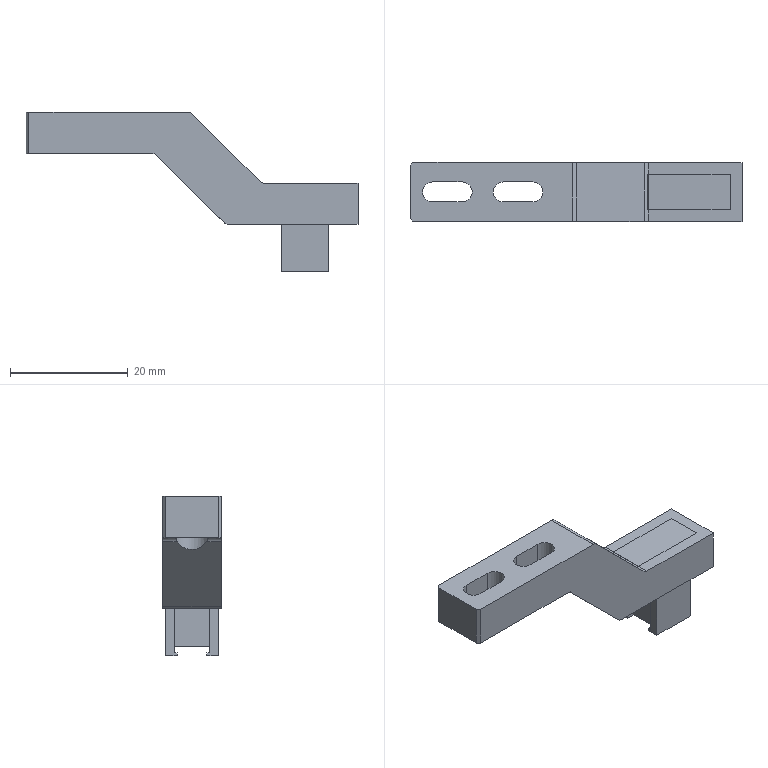NC program | NX | posted with a generic post | part box 56.3 x 10 x 27 mm
Lines 2775 to 3642 of 5717:
(ZLEVEL_PROFILE_COPY_2 , TOOL : D2)
N5506 T02 M6
N5508 G54
N5510 G17 G0 G90 X-11.938 Y0.7 S9500 M3
N5512 G43 Z30. H2
N5514 Z1.5
N5516 G94 G1 X-12.439 Z1.474 F800.
N5518 X-12.69 Y0.606 Z1.46
N5520 X-12.889 Y0.425 Z1.446
N5522 X-12.997 Y0.214 Z1.433
N5524 X-13.025 Y-0.086 Z1.417
N5526 X-12.926 Y-0.37 Z1.402
N5528 X-12.718 Y-0.588 Z1.386
N5530 X-12.439 Y-0.7 Z1.37
N5532 X-7.244 Z1.098
N5534 X-7.053 Y-0.658 Z1.088
N5536 X-6.815 Y-0.499 Z1.073
N5538 X-6.659 Y-0.259 Z1.058
N5540 X-6.611 Y0.023 Z1.043
N5542 X-6.678 Y0.302 Z1.028
N5544 X-6.813 Y0.497 Z1.015
N5546 X-6.991 Y0.629 Z1.003
N5548 X-7.202 Y0.7 Z0.992
N5550 X-12.439 Z0.717
N5552 X-12.69 Y0.606 Z0.703
N5554 X-12.889 Y0.425 Z0.689
N5556 X-12.997 Y0.214 Z0.677
N5558 X-13.025 Y-0.086 Z0.661
N5560 X-12.926 Y-0.37 Z0.645
N5562 X-12.718 Y-0.588 Z0.629
N5564 X-12.439 Y-0.7 Z0.614
N5566 X-7.244 Z0.341
N5568 X-7.053 Y-0.658 Z0.331
N5570 X-6.815 Y-0.499 Z0.316
N5572 X-6.659 Y-0.259 Z0.301
N5574 X-6.611 Y0.023 Z0.286
N5576 X-6.678 Y0.302 Z0.271
N5578 X-6.813 Y0.497 Z0.259
N5580 X-6.991 Y0.629 Z0.247
N5582 X-7.202 Y0.7 Z0.235
N5584 X-12.439 Z-0.039
N5586 X-12.69 Y0.606 Z-0.053
N5588 X-12.889 Y0.425 Z-0.067
N5590 X-12.997 Y0.214 Z-0.08
N5592 X-13.025 Y-0.086 Z-0.095
N5594 X-12.926 Y-0.37 Z-0.111
N5596 X-12.718 Y-0.588 Z-0.127
N5598 X-12.439 Y-0.7 Z-0.143
N5600 X-12.32 Z-0.149
N5602 X-7.32 F1100.
N5604 G3 X-6.62 Y0. R0.7
N5606 X-7.32 Y0.7 R0.7
N5608 G1 X-12.32
N5610 G3 X-13.02 Y0. R0.7
N5612 X-12.32 Y-0.7 R0.7
N5614 G1 X-7.359 Z-0.236
N5616 X-7.226 Y-0.686 Z-0.238
N5618 X-7.164 Y-0.676 Z-0.239
N5620 X-7.061 Y-0.643 Z-0.241
N5622 X-6.982 Y-0.604 Z-0.242
N5624 X-6.888 Y-0.541 Z-0.244
N5626 X-6.826 Y-0.485 Z-0.246
N5628 X-6.755 Y-0.399 Z-0.248
N5630 X-6.709 Y-0.328 Z-0.249
N5632 X-6.656 Y-0.221 Z-0.251
N5634 X-6.636 Y-0.146 Z-0.253
N5636 X-6.622 Y0.052 Z-0.256
N5638 X-6.642 Y0.173 Z-0.258
N5640 X-6.671 Y0.242 Z-0.26
N5642 X-6.735 Y0.373 Z-0.262
N5644 X-6.765 Y0.414 Z-0.263
N5646 X-6.853 Y0.511 Z-0.266
N5648 X-6.902 Y0.554 Z-0.267
N5650 X-6.994 Y0.612 Z-0.269
N5652 X-7.074 Y0.647 Z-0.27
N5654 X-7.161 Y0.675 Z-0.272
N5656 X-7.265 Y0.69 Z-0.274
N5658 X-7.364 Y0.7 Z-0.275
N5660 X-7.463 Z-0.277
N5662 X-8.654 Z-0.298
N5664 X-12.32
N5666 G3 X-13.02 Y0. R0.7
N5668 X-12.32 Y-0.7 R0.7
N5670 G1 X-7.359 Z-0.384
N5672 X-7.226 Y-0.686 Z-0.387
N5674 X-7.164 Y-0.676 Z-0.388
N5676 X-7.061 Y-0.643 Z-0.39
N5678 X-6.982 Y-0.604 Z-0.391
N5680 X-6.888 Y-0.541 Z-0.393
N5682 X-6.826 Y-0.485 Z-0.395
N5684 X-6.755 Y-0.399 Z-0.397
N5686 X-6.709 Y-0.328 Z-0.398
N5688 X-6.656 Y-0.221 Z-0.4
N5690 X-6.636 Y-0.146 Z-0.402
N5692 X-6.622 Y0.052 Z-0.405
N5694 X-6.642 Y0.173 Z-0.407
N5696 X-6.671 Y0.242 Z-0.409
N5698 X-6.735 Y0.373 Z-0.411
N5700 X-6.765 Y0.414 Z-0.412
N5702 X-6.853 Y0.511 Z-0.414
N5704 X-6.902 Y0.554 Z-0.416
N5706 X-6.994 Y0.612 Z-0.418
N5708 X-7.074 Y0.647 Z-0.419
N5710 X-7.161 Y0.675 Z-0.421
N5712 X-7.265 Y0.69 Z-0.423
N5714 X-7.364 Y0.7 Z-0.424
N5716 X-7.463 Z-0.426
N5718 X-8.654 Z-0.447
N5720 X-12.32
N5722 G3 X-13.02 Y0. R0.7
N5724 X-12.32 Y-0.7 R0.7
N5726 G1 X-7.359 Z-0.533
N5728 X-7.226 Y-0.686 Z-0.536
N5730 X-7.164 Y-0.676 Z-0.537
N5732 X-7.061 Y-0.643 Z-0.539
N5734 X-6.982 Y-0.604 Z-0.54
N5736 X-6.888 Y-0.541 Z-0.542
N5738 X-6.826 Y-0.485 Z-0.544
N5740 X-6.755 Y-0.399 Z-0.546
N5742 X-6.709 Y-0.328 Z-0.547
N5744 X-6.656 Y-0.221 Z-0.549
N5746 X-6.636 Y-0.146 Z-0.551
N5748 X-6.622 Y0.052 Z-0.554
N5750 X-6.642 Y0.173 Z-0.556
N5752 X-6.671 Y0.242 Z-0.558
N5754 X-6.735 Y0.373 Z-0.56
N5756 X-6.765 Y0.414 Z-0.561
N5758 X-6.853 Y0.511 Z-0.563
N5760 X-6.902 Y0.554 Z-0.565
N5762 X-6.994 Y0.612 Z-0.566
N5764 X-7.074 Y0.647 Z-0.568
N5766 X-7.161 Y0.675 Z-0.57
N5768 X-7.265 Y0.69 Z-0.572
N5770 X-7.364 Y0.7 Z-0.573
N5772 X-7.463 Z-0.575
N5774 X-8.654 Z-0.596
N5776 X-12.32
N5778 G3 X-13.02 Y0. R0.7
N5780 X-12.32 Y-0.7 R0.7
N5782 G1 X-7.359 Z-0.682
N5784 X-7.226 Y-0.686 Z-0.685
N5786 X-7.164 Y-0.676 Z-0.686
N5788 X-7.061 Y-0.643 Z-0.688
N5790 X-6.982 Y-0.604 Z-0.689
N5792 X-6.888 Y-0.541 Z-0.691
N5794 X-6.826 Y-0.485 Z-0.693
N5796 X-6.755 Y-0.399 Z-0.695
N5798 X-6.709 Y-0.328 Z-0.696
N5800 X-6.656 Y-0.221 Z-0.698
N5802 X-6.636 Y-0.146 Z-0.7
N5804 X-6.622 Y0.052 Z-0.703
N5806 X-6.642 Y0.173 Z-0.705
N5808 X-6.671 Y0.242 Z-0.707
N5810 X-6.735 Y0.373 Z-0.709
N5812 X-6.765 Y0.414 Z-0.71
N5814 X-6.853 Y0.511 Z-0.712
N5816 X-6.902 Y0.554 Z-0.714
N5818 X-6.994 Y0.612 Z-0.715
N5820 X-7.074 Y0.647 Z-0.717
N5822 X-7.161 Y0.675 Z-0.719
N5824 X-7.265 Y0.69 Z-0.72
N5826 X-7.364 Y0.7 Z-0.722
N5828 X-7.463 Z-0.724
N5830 X-8.654 Z-0.745
N5832 X-12.32
N5834 G3 X-13.02 Y0. R0.7
N5836 X-12.32 Y-0.7 R0.7
N5838 G1 X-7.359 Z-0.831
N5840 X-7.226 Y-0.686 Z-0.834
N5842 X-7.164 Y-0.676 Z-0.835
N5844 X-7.061 Y-0.643 Z-0.837
N5846 X-6.982 Y-0.604 Z-0.838
N5848 X-6.888 Y-0.541 Z-0.84
N5850 X-6.826 Y-0.485 Z-0.842
N5852 X-6.755 Y-0.399 Z-0.844
N5854 X-6.709 Y-0.328 Z-0.845
N5856 X-6.656 Y-0.221 Z-0.847
N5858 X-6.636 Y-0.146 Z-0.849
N5860 X-6.622 Y0.052 Z-0.852
N5862 X-6.642 Y0.173 Z-0.854
N5864 X-6.671 Y0.242 Z-0.856
N5866 X-6.735 Y0.373 Z-0.858
N5868 X-6.765 Y0.414 Z-0.859
N5870 X-6.853 Y0.511 Z-0.861
N5872 X-6.902 Y0.554 Z-0.862
N5874 X-6.994 Y0.612 Z-0.864
N5876 X-7.074 Y0.647 Z-0.866
N5878 X-7.161 Y0.675 Z-0.868
N5880 X-7.265 Y0.69 Z-0.869
N5882 X-7.364 Y0.7 Z-0.871
N5884 X-7.463 Z-0.873
N5886 X-8.654 Z-0.894
N5888 X-12.32
N5890 G3 X-13.02 Y0. R0.7
N5892 X-12.32 Y-0.7 R0.7
N5894 G1 X-7.359 Z-0.98
N5896 X-7.226 Y-0.686 Z-0.983
N5898 X-7.164 Y-0.676 Z-0.984
N5900 X-7.061 Y-0.643 Z-0.986
N5902 X-6.982 Y-0.604 Z-0.987
N5904 X-6.888 Y-0.541 Z-0.989
N5906 X-6.826 Y-0.485 Z-0.991
N5908 X-6.755 Y-0.399 Z-0.993
N5910 X-6.709 Y-0.328 Z-0.994
N5912 X-6.656 Y-0.221 Z-0.996
N5914 X-6.636 Y-0.146 Z-0.998
N5916 X-6.622 Y0.052 Z-1.001
N5918 X-6.642 Y0.173 Z-1.003
N5920 X-6.671 Y0.242 Z-1.004
N5922 X-6.735 Y0.373 Z-1.007
N5924 X-6.765 Y0.414 Z-1.008
N5926 X-6.853 Y0.511 Z-1.01
N5928 X-6.902 Y0.554 Z-1.011
N5930 X-6.994 Y0.612 Z-1.013
N5932 X-7.074 Y0.647 Z-1.015
N5934 X-7.161 Y0.675 Z-1.016
N5936 X-7.265 Y0.69 Z-1.018
N5938 X-7.364 Y0.7 Z-1.02
N5940 X-7.463 Z-1.022
N5942 X-8.654 Z-1.043
N5944 X-12.32
N5946 G3 X-13.02 Y0. R0.7
N5948 X-12.32 Y-0.7 R0.7
N5950 G1 X-7.359 Z-1.129
N5952 X-7.226 Y-0.686 Z-1.131
N5954 X-7.164 Y-0.676 Z-1.133
N5956 X-7.061 Y-0.643 Z-1.135
N5958 X-6.982 Y-0.604 Z-1.136
N5960 X-6.888 Y-0.541 Z-1.138
N5962 X-6.826 Y-0.485 Z-1.14
N5964 X-6.755 Y-0.399 Z-1.142
N5966 X-6.709 Y-0.328 Z-1.143
N5968 X-6.656 Y-0.221 Z-1.145
N5970 X-6.636 Y-0.146 Z-1.146
N5972 X-6.622 Y0.052 Z-1.15
N5974 X-6.642 Y0.173 Z-1.152
N5976 X-6.671 Y0.242 Z-1.153
N5978 X-6.735 Y0.373 Z-1.156
N5980 X-6.765 Y0.414 Z-1.157
N5982 X-6.853 Y0.511 Z-1.159
N5984 X-6.902 Y0.554 Z-1.16
N5986 X-6.994 Y0.612 Z-1.162
N5988 X-7.074 Y0.647 Z-1.164
N5990 X-7.161 Y0.675 Z-1.165
N5992 X-7.265 Y0.69 Z-1.167
N5994 X-7.364 Y0.7 Z-1.169
N5996 X-7.463 Z-1.171
N5998 X-8.654 Z-1.191
N6000 X-12.32
N6002 G3 X-13.02 Y0. R0.7
N6004 X-12.32 Y-0.7 R0.7
N6006 G1 X-7.359 Z-1.278
N6008 X-7.226 Y-0.686 Z-1.28
N6010 X-7.164 Y-0.676 Z-1.282
N6012 X-7.061 Y-0.643 Z-1.283
N6014 X-6.982 Y-0.604 Z-1.285
N6016 X-6.888 Y-0.541 Z-1.287
N6018 X-6.826 Y-0.485 Z-1.288
N6020 X-6.755 Y-0.399 Z-1.29
N6022 X-6.709 Y-0.328 Z-1.292
N6024 X-6.656 Y-0.221 Z-1.294
N6026 X-6.636 Y-0.146 Z-1.295
N6028 X-6.622 Y0.052 Z-1.299
N6030 X-6.642 Y0.173 Z-1.301
N6032 X-6.671 Y0.242 Z-1.302
N6034 X-6.735 Y0.373 Z-1.305
N6036 X-6.765 Y0.414 Z-1.306
N6038 X-6.853 Y0.511 Z-1.308
N6040 X-6.902 Y0.554 Z-1.309
N6042 X-6.994 Y0.612 Z-1.311
N6044 X-7.074 Y0.647 Z-1.313
N6046 X-7.161 Y0.675 Z-1.314
N6048 X-7.265 Y0.69 Z-1.316
N6050 X-7.364 Y0.7 Z-1.318
N6052 X-7.463 Z-1.32
N6054 X-8.654 Z-1.34
N6056 X-12.32
N6058 G3 X-13.02 Y0. R0.7
N6060 X-12.32 Y-0.7 R0.7
N6062 G1 X-7.359 Z-1.427
N6064 X-7.226 Y-0.686 Z-1.429
N6066 X-7.164 Y-0.676 Z-1.43
N6068 X-7.061 Y-0.643 Z-1.432
N6070 X-6.982 Y-0.604 Z-1.434
N6072 X-6.888 Y-0.541 Z-1.436
N6074 X-6.826 Y-0.485 Z-1.437
N6076 X-6.755 Y-0.399 Z-1.439
N6078 X-6.709 Y-0.328 Z-1.441
N6080 X-6.656 Y-0.221 Z-1.443
N6082 X-6.636 Y-0.146 Z-1.444
N6084 X-6.622 Y0.052 Z-1.448
N6086 X-6.642 Y0.173 Z-1.45
N6088 X-6.671 Y0.242 Z-1.451
N6090 X-6.735 Y0.373 Z-1.454
N6092 X-6.765 Y0.414 Z-1.455
N6094 X-6.853 Y0.511 Z-1.457
N6096 X-6.902 Y0.554 Z-1.458
N6098 X-6.994 Y0.612 Z-1.46
N6100 X-7.074 Y0.647 Z-1.462
N6102 X-7.161 Y0.675 Z-1.463
N6104 X-7.265 Y0.69 Z-1.465
N6106 X-7.364 Y0.7 Z-1.467
N6108 X-7.463 Z-1.469
N6110 X-8.654 Z-1.489
N6112 X-12.32
N6114 G3 X-13.02 Y0. R0.7
N6116 X-12.32 Y-0.7 R0.7
N6118 G1 X-7.359 Z-1.576
N6120 X-7.226 Y-0.686 Z-1.578
N6122 X-7.164 Y-0.676 Z-1.579
N6124 X-7.061 Y-0.643 Z-1.581
N6126 X-6.982 Y-0.604 Z-1.583
N6128 X-6.888 Y-0.541 Z-1.585
N6130 X-6.826 Y-0.485 Z-1.586
N6132 X-6.755 Y-0.399 Z-1.588
N6134 X-6.709 Y-0.328 Z-1.59
N6136 X-6.656 Y-0.221 Z-1.592
N6138 X-6.636 Y-0.146 Z-1.593
N6140 X-6.622 Y0.052 Z-1.597
N6142 X-6.642 Y0.173 Z-1.599
N6144 X-6.671 Y0.242 Z-1.6
N6146 X-6.735 Y0.373 Z-1.603
N6148 X-6.765 Y0.414 Z-1.604
N6150 X-6.853 Y0.511 Z-1.606
N6152 X-6.902 Y0.554 Z-1.607
N6154 X-6.994 Y0.612 Z-1.609
N6156 X-7.074 Y0.647 Z-1.611
N6158 X-7.161 Y0.675 Z-1.612
N6160 X-7.265 Y0.69 Z-1.614
N6162 X-7.364 Y0.7 Z-1.616
N6164 X-7.463 Z-1.618
N6166 X-8.654 Z-1.638
N6168 X-12.32
N6170 G3 X-13.02 Y0. R0.7
N6172 X-12.32 Y-0.7 R0.7
N6174 G1 X-7.359 Z-1.725
N6176 X-7.226 Y-0.686 Z-1.727
N6178 X-7.164 Y-0.676 Z-1.728
N6180 X-7.061 Y-0.643 Z-1.73
N6182 X-6.982 Y-0.604 Z-1.732
N6184 X-6.888 Y-0.541 Z-1.734
N6186 X-6.826 Y-0.485 Z-1.735
N6188 X-6.755 Y-0.399 Z-1.737
N6190 X-6.709 Y-0.328 Z-1.739
N6192 X-6.656 Y-0.221 Z-1.741
N6194 X-6.636 Y-0.146 Z-1.742
N6196 X-6.622 Y0.052 Z-1.746
N6198 X-6.642 Y0.173 Z-1.748
N6200 X-6.671 Y0.242 Z-1.749
N6202 X-6.735 Y0.373 Z-1.752
N6204 X-6.765 Y0.414 Z-1.753
N6206 X-6.853 Y0.511 Z-1.755
N6208 X-6.902 Y0.554 Z-1.756
N6210 X-6.994 Y0.612 Z-1.758
N6212 X-7.074 Y0.647 Z-1.76
N6214 X-7.161 Y0.675 Z-1.761
N6216 X-7.265 Y0.69 Z-1.763
N6218 X-7.364 Y0.7 Z-1.765
N6220 X-7.463 Z-1.766
N6222 X-8.654 Z-1.787
N6224 X-12.32
N6226 G3 X-13.02 Y0. R0.7
N6228 X-12.32 Y-0.7 R0.7
N6230 G1 X-7.359 Z-1.874
N6232 X-7.226 Y-0.686 Z-1.876
N6234 X-7.164 Y-0.676 Z-1.877
N6236 X-7.061 Y-0.643 Z-1.879
N6238 X-6.982 Y-0.604 Z-1.881
N6240 X-6.888 Y-0.541 Z-1.883
N6242 X-6.826 Y-0.485 Z-1.884
N6244 X-6.755 Y-0.399 Z-1.886
N6246 X-6.709 Y-0.328 Z-1.888
N6248 X-6.656 Y-0.221 Z-1.89
N6250 X-6.636 Y-0.146 Z-1.891
N6252 X-6.622 Y0.052 Z-1.895
N6254 X-6.642 Y0.173 Z-1.897
N6256 X-6.671 Y0.242 Z-1.898
N6258 X-6.735 Y0.373 Z-1.901
N6260 X-6.765 Y0.414 Z-1.902
N6262 X-6.853 Y0.511 Z-1.904
N6264 X-6.902 Y0.554 Z-1.905
N6266 X-6.994 Y0.612 Z-1.907
N6268 X-7.074 Y0.647 Z-1.908
N6270 X-7.161 Y0.675 Z-1.91
N6272 X-7.265 Y0.69 Z-1.912
N6274 X-7.364 Y0.7 Z-1.914
N6276 X-7.463 Z-1.915
N6278 X-8.654 Z-1.936
N6280 X-12.32
N6282 G3 X-13.02 Y0. R0.7
N6284 X-12.32 Y-0.7 R0.7
N6286 G1 X-7.359 Z-2.023
N6288 X-7.226 Y-0.686 Z-2.025
N6290 X-7.164 Y-0.676 Z-2.026
N6292 X-7.061 Y-0.643 Z-2.028
N6294 X-6.982 Y-0.604 Z-2.03
N6296 X-6.888 Y-0.541 Z-2.032
N6298 X-6.826 Y-0.485 Z-2.033
N6300 X-6.755 Y-0.399 Z-2.035
N6302 X-6.709 Y-0.328 Z-2.037
N6304 X-6.656 Y-0.221 Z-2.039
N6306 X-6.636 Y-0.146 Z-2.04
N6308 X-6.622 Y0.052 Z-2.044
N6310 X-6.642 Y0.173 Z-2.046
N6312 X-6.671 Y0.242 Z-2.047
N6314 X-6.735 Y0.373 Z-2.05
N6316 X-6.765 Y0.414
N6318 X-6.853 Y0.511 Z-2.053
N6320 X-6.902 Y0.554 Z-2.054
N6322 X-6.994 Y0.612 Z-2.056
N6324 X-7.074 Y0.647 Z-2.057
N6326 X-7.161 Y0.675 Z-2.059
N6328 X-7.265 Y0.69 Z-2.061
N6330 X-7.364 Y0.7 Z-2.063
N6332 X-7.463 Z-2.064
N6334 X-8.654 Z-2.085
N6336 X-12.32
N6338 G3 X-13.02 Y0. R0.7
N6340 X-12.32 Y-0.7 R0.7
N6342 G1 X-7.359 Z-2.172
N6344 X-7.226 Y-0.686 Z-2.174
N6346 X-7.164 Y-0.676 Z-2.175
N6348 X-7.061 Y-0.643 Z-2.177
N6350 X-6.982 Y-0.604 Z-2.179
N6352 X-6.888 Y-0.541 Z-2.181
N6354 X-6.826 Y-0.485 Z-2.182
N6356 X-6.755 Y-0.399 Z-2.184
N6358 X-6.709 Y-0.328 Z-2.186
N6360 X-6.656 Y-0.221 Z-2.188
N6362 X-6.636 Y-0.146 Z-2.189
N6364 X-6.622 Y0.052 Z-2.192
N6366 X-6.642 Y0.173 Z-2.195
N6368 X-6.671 Y0.242 Z-2.196
N6370 X-6.735 Y0.373 Z-2.198
N6372 X-6.765 Y0.414 Z-2.199
N6374 X-6.853 Y0.511 Z-2.202
N6376 X-6.902 Y0.554 Z-2.203
N6378 X-6.994 Y0.612 Z-2.205
N6380 X-7.074 Y0.647 Z-2.206
N6382 X-7.161 Y0.675 Z-2.208
N6384 X-7.265 Y0.69 Z-2.21
N6386 X-7.364 Y0.7 Z-2.212
N6388 X-7.463 Z-2.213
N6390 X-8.654 Z-2.234
N6392 X-12.32
N6394 G3 X-13.02 Y0. R0.7
N6396 X-12.32 Y-0.7 R0.7
N6398 G1 X-7.359 Z-2.321
N6400 X-7.226 Y-0.686 Z-2.323
N6402 X-7.164 Y-0.676 Z-2.324
N6404 X-7.061 Y-0.643 Z-2.326
N6406 X-6.982 Y-0.604 Z-2.328
N6408 X-6.888 Y-0.541 Z-2.33
N6410 X-6.826 Y-0.485 Z-2.331
N6412 X-6.755 Y-0.399 Z-2.333
N6414 X-6.709 Y-0.328 Z-2.334
N6416 X-6.656 Y-0.221 Z-2.337
N6418 X-6.636 Y-0.146 Z-2.338
N6420 X-6.622 Y0.052 Z-2.341
N6422 X-6.642 Y0.173 Z-2.344
N6424 X-6.671 Y0.242 Z-2.345
N6426 X-6.735 Y0.373 Z-2.347
N6428 X-6.765 Y0.414 Z-2.348
N6430 X-6.853 Y0.511 Z-2.351
N6432 X-6.902 Y0.554 Z-2.352
N6434 X-6.994 Y0.612 Z-2.354
N6436 X-7.074 Y0.647 Z-2.355
N6438 X-7.161 Y0.675 Z-2.357
N6440 X-7.265 Y0.69 Z-2.359
N6442 X-7.364 Y0.7 Z-2.36
N6444 X-7.463 Z-2.362
N6446 X-8.654 Z-2.383
N6448 X-12.32
N6450 G3 X-13.02 Y0. R0.7
N6452 X-12.32 Y-0.7 R0.7
N6454 G1 X-7.359 Z-2.47
N6456 X-7.226 Y-0.686 Z-2.472
N6458 X-7.164 Y-0.676 Z-2.473
N6460 X-7.061 Y-0.643 Z-2.475
N6462 X-6.982 Y-0.604 Z-2.476
N6464 X-6.888 Y-0.541 Z-2.478
N6466 X-6.826 Y-0.485 Z-2.48
N6468 X-6.755 Y-0.399 Z-2.482
N6470 X-6.709 Y-0.328 Z-2.483
N6472 X-6.656 Y-0.221 Z-2.486
N6474 X-6.636 Y-0.146 Z-2.487
N6476 X-6.622 Y0.052 Z-2.49
N6478 X-6.642 Y0.173 Z-2.493
N6480 X-6.671 Y0.242 Z-2.494
N6482 X-6.735 Y0.373 Z-2.496
N6484 X-6.765 Y0.414 Z-2.497
N6486 X-6.853 Y0.511 Z-2.5
N6488 X-6.902 Y0.554 Z-2.501
N6490 X-6.994 Y0.612 Z-2.503
N6492 X-7.074 Y0.647 Z-2.504
N6494 X-7.161 Y0.675 Z-2.506
N6496 X-7.265 Y0.69 Z-2.508
N6498 X-7.364 Y0.7 Z-2.509
N6500 X-7.463 Z-2.511
N6502 X-8.654 Z-2.532
N6504 X-12.32
N6506 G3 X-13.02 Y0. R0.7
N6508 X-12.32 Y-0.7 R0.7
N6510 G1 X-7.359 Z-2.619
N6512 X-7.226 Y-0.686 Z-2.621
N6514 X-7.164 Y-0.676 Z-2.622
N6516 X-7.061 Y-0.643 Z-2.624
N6518 X-6.982 Y-0.604 Z-2.625
N6520 X-6.888 Y-0.541 Z-2.627
N6522 X-6.826 Y-0.485 Z-2.629
N6524 X-6.755 Y-0.399 Z-2.631
N6526 X-6.709 Y-0.328 Z-2.632
N6528 X-6.656 Y-0.221 Z-2.634
N6530 X-6.636 Y-0.146 Z-2.636
N6532 X-6.622 Y0.052 Z-2.639
N6534 X-6.642 Y0.173 Z-2.641
N6536 X-6.671 Y0.242 Z-2.643
N6538 X-6.735 Y0.373 Z-2.645
N6540 X-6.765 Y0.414 Z-2.646
N6542 X-6.853 Y0.511 Z-2.649
N6544 X-6.902 Y0.554 Z-2.65
N6546 X-6.994 Y0.612 Z-2.652
N6548 X-7.074 Y0.647 Z-2.653
N6550 X-7.161 Y0.675 Z-2.655
N6552 X-7.265 Y0.69 Z-2.657
N6554 X-7.364 Y0.7 Z-2.658
N6556 X-7.463 Z-2.66
N6558 X-8.654 Z-2.681
N6560 X-12.32
N6562 G3 X-13.02 Y0. R0.7
N6564 X-12.32 Y-0.7 R0.7
N6566 G1 X-7.359 Z-2.767
N6568 X-7.226 Y-0.686 Z-2.77
N6570 X-7.164 Y-0.676 Z-2.771
N6572 X-7.061 Y-0.643 Z-2.773
N6574 X-6.982 Y-0.604 Z-2.774
N6576 X-6.888 Y-0.541 Z-2.776
N6578 X-6.826 Y-0.485 Z-2.778
N6580 X-6.755 Y-0.399 Z-2.78
N6582 X-6.709 Y-0.328 Z-2.781
N6584 X-6.656 Y-0.221 Z-2.783
N6586 X-6.636 Y-0.146 Z-2.785
N6588 X-6.622 Y0.052 Z-2.788
N6590 X-6.642 Y0.173 Z-2.79
N6592 X-6.671 Y0.242 Z-2.792
N6594 X-6.735 Y0.373 Z-2.794
N6596 X-6.765 Y0.414 Z-2.795
N6598 X-6.853 Y0.511 Z-2.797
N6600 X-6.902 Y0.554 Z-2.799
N6602 X-6.994 Y0.612 Z-2.801
N6604 X-7.074 Y0.647 Z-2.802
N6606 X-7.161 Y0.675 Z-2.804
N6608 X-7.265 Y0.69 Z-2.806
N6610 X-7.364 Y0.7 Z-2.807
N6612 X-7.463 Z-2.809
N6614 X-8.654 Z-2.83
N6616 X-12.32
N6618 G3 X-13.02 Y0. R0.7
N6620 X-12.32 Y-0.7 R0.7
N6622 G1 X-7.359 Z-2.916
N6624 X-7.226 Y-0.686 Z-2.919
N6626 X-7.164 Y-0.676 Z-2.92
N6628 X-7.061 Y-0.643 Z-2.922
N6630 X-6.982 Y-0.604 Z-2.923
N6632 X-6.888 Y-0.541 Z-2.925
N6634 X-6.826 Y-0.485 Z-2.927
N6636 X-6.755 Y-0.399 Z-2.929
N6638 X-6.709 Y-0.328 Z-2.93
N6640 X-6.656 Y-0.221 Z-2.932
N6642 X-6.636 Y-0.146 Z-2.934
N6644 X-6.622 Y0.052 Z-2.937
N6646 X-6.642 Y0.173 Z-2.939
N6648 X-6.671 Y0.242 Z-2.941
N6650 X-6.735 Y0.373 Z-2.943
N6652 X-6.765 Y0.414 Z-2.944
N6654 X-6.853 Y0.511 Z-2.946
N6656 X-6.902 Y0.554 Z-2.948
N6658 X-6.994 Y0.612 Z-2.949
N6660 X-7.074 Y0.647 Z-2.951
N6662 X-7.161 Y0.675 Z-2.953
N6664 X-7.265 Y0.69 Z-2.954
N6666 X-7.364 Y0.7 Z-2.956
N6668 X-7.463 Z-2.958
N6670 X-8.654 Z-2.979
N6672 X-12.32
N6674 G3 X-13.02 Y0. R0.7
N6676 X-12.32 Y-0.7 R0.7
N6678 G1 X-7.359 Z-3.065
N6680 X-7.226 Y-0.686 Z-3.068
N6682 X-7.164 Y-0.676 Z-3.069
N6684 X-7.061 Y-0.643 Z-3.071
N6686 X-6.982 Y-0.604 Z-3.072
N6688 X-6.888 Y-0.541 Z-3.074
N6690 X-6.826 Y-0.485 Z-3.076
N6692 X-6.755 Y-0.399 Z-3.078
N6694 X-6.709 Y-0.328 Z-3.079
N6696 X-6.656 Y-0.221 Z-3.081
N6698 X-6.636 Y-0.146 Z-3.083
N6700 X-6.622 Y0.052 Z-3.086
N6702 X-6.642 Y0.173 Z-3.088
N6704 X-6.671 Y0.242 Z-3.09
N6706 X-6.735 Y0.373 Z-3.092
N6708 X-6.765 Y0.414 Z-3.093
N6710 X-6.853 Y0.511 Z-3.095
N6712 X-6.902 Y0.554 Z-3.096
N6714 X-6.994 Y0.612 Z-3.098
N6716 X-7.074 Y0.647 Z-3.1
N6718 X-7.161 Y0.675 Z-3.102
N6720 X-7.265 Y0.69 Z-3.103
N6722 X-7.364 Y0.7 Z-3.105
N6724 X-7.463 Z-3.107
N6726 X-8.654 Z-3.128
N6728 X-12.32
N6730 G3 X-13.02 Y0. R0.7
N6732 X-12.32 Y-0.7 R0.7
N6734 G1 X-7.359 Z-3.214
N6736 X-7.226 Y-0.686 Z-3.217
N6738 X-7.164 Y-0.676 Z-3.218
N6740 X-7.061 Y-0.643 Z-3.22
N6742 X-6.982 Y-0.604 Z-3.221
N6744 X-6.888 Y-0.541 Z-3.223
N6746 X-6.826 Y-0.485 Z-3.225
N6748 X-6.755 Y-0.399 Z-3.227
N6750 X-6.709 Y-0.328 Z-3.228
N6752 X-6.656 Y-0.221 Z-3.23
N6754 X-6.636 Y-0.146 Z-3.232
N6756 X-6.622 Y0.052 Z-3.235
N6758 X-6.642 Y0.173 Z-3.237
N6760 X-6.671 Y0.242 Z-3.238
N6762 X-6.735 Y0.373 Z-3.241
N6764 X-6.765 Y0.414 Z-3.242
N6766 X-6.853 Y0.511 Z-3.244
N6768 X-6.902 Y0.554 Z-3.245
N6770 X-6.994 Y0.612 Z-3.247
N6772 X-7.074 Y0.647 Z-3.249
N6774 X-7.161 Y0.675 Z-3.25
N6776 X-7.265 Y0.69 Z-3.252
N6778 X-7.364 Y0.7 Z-3.254
N6780 X-7.463 Z-3.256
N6782 X-8.654 Z-3.277
N6784 X-12.32
N6786 G3 X-13.02 Y0. R0.7
N6788 X-12.32 Y-0.7 R0.7
N6790 G1 X-7.359 Z-3.363
N6792 X-7.226 Y-0.686 Z-3.366
N6794 X-7.164 Y-0.676 Z-3.367
N6796 X-7.061 Y-0.643 Z-3.369
N6798 X-6.982 Y-0.604 Z-3.37
N6800 X-6.888 Y-0.541 Z-3.372
N6802 X-6.826 Y-0.485 Z-3.374
N6804 X-6.755 Y-0.399 Z-3.376
N6806 X-6.709 Y-0.328 Z-3.377
N6808 X-6.656 Y-0.221 Z-3.379
N6810 X-6.636 Y-0.146 Z-3.381
N6812 X-6.622 Y0.052 Z-3.384
N6814 X-6.642 Y0.173 Z-3.386
N6816 X-6.671 Y0.242 Z-3.387
N6818 X-6.735 Y0.373 Z-3.39
N6820 X-6.765 Y0.414 Z-3.391
N6822 X-6.853 Y0.511 Z-3.393
N6824 X-6.902 Y0.554 Z-3.394
N6826 X-6.994 Y0.612 Z-3.396
N6828 X-7.074 Y0.647 Z-3.398
N6830 X-7.161 Y0.675 Z-3.399
N6832 X-7.265 Y0.69 Z-3.401
N6834 X-7.364 Y0.7 Z-3.403
N6836 X-7.463 Z-3.405
N6838 X-8.654 Z-3.426
N6840 X-12.32
N6842 G3 X-13.02 Y0. R0.7
N6844 X-12.32 Y-0.7 R0.7
N6846 G1 X-7.359 Z-3.512
N6848 X-7.226 Y-0.686 Z-3.514
N6850 X-7.164 Y-0.676 Z-3.516
N6852 X-7.061 Y-0.643 Z-3.517
N6854 X-6.982 Y-0.604 Z-3.519
N6856 X-6.888 Y-0.541 Z-3.521
N6858 X-6.826 Y-0.485 Z-3.523
N6860 X-6.755 Y-0.399 Z-3.524
N6862 X-6.709 Y-0.328 Z-3.526
N6864 X-6.656 Y-0.221 Z-3.528
N6866 X-6.636 Y-0.146 Z-3.529
N6868 X-6.622 Y0.052 Z-3.533
N6870 X-6.642 Y0.173 Z-3.535
N6872 X-6.671 Y0.242 Z-3.536
N6874 X-6.735 Y0.373 Z-3.539
N6876 X-6.765 Y0.414 Z-3.54
N6878 X-6.853 Y0.511 Z-3.542
N6880 X-6.902 Y0.554 Z-3.543
N6882 X-6.994 Y0.612 Z-3.545
N6884 X-7.074 Y0.647 Z-3.547
N6886 X-7.161 Y0.675 Z-3.548
N6888 X-7.265 Y0.69 Z-3.55
N6890 X-7.364 Y0.7 Z-3.552
N6892 X-7.463 Z-3.554
N6894 X-8.654 Z-3.574
N6896 X-12.32
N6898 G3 X-13.02 Y0. R0.7
N6900 X-12.32 Y-0.7 R0.7
N6902 G1 X-7.359 Z-3.661
N6904 X-7.226 Y-0.686 Z-3.663
N6906 X-7.164 Y-0.676 Z-3.665
N6908 X-7.061 Y-0.643 Z-3.666
N6910 X-6.982 Y-0.604 Z-3.668
N6912 X-6.888 Y-0.541 Z-3.67
N6914 X-6.826 Y-0.485 Z-3.671
N6916 X-6.751 Y-0.394 Z-3.674
N6918 X-6.709 Y-0.328 Z-3.675
N6920 X-6.666 Y-0.233 Z-3.677
N6922 X-6.643 Y-0.144 Z-3.678
N6924 X-6.629 Y-0.022 Z-3.681
N6926 X-6.628 Y0.051 Z-3.682
N6928 X-6.647 Y0.156 Z-3.684
N6930 X-6.671 Y0.242 Z-3.685
N6932 X-6.715 Y0.343 Z-3.687
N6934 X-6.765 Y0.414 Z-3.689
N6936 X-6.85 Y0.508 Z-3.691
N6938 X-6.902 Y0.554 Z-3.692
N6940 X-6.993 Y0.611 Z-3.694
N6942 X-7.074 Y0.647 Z-3.696
N6944 X-7.161 Y0.675 Z-3.697
N6946 X-7.265 Y0.69 Z-3.699
N6948 X-7.364 Y0.7 Z-3.701
N6950 X-7.463 Z-3.703
N6952 X-8.654 Z-3.723
N6954 X-12.32
N6956 G3 X-13.02 Y0. R0.7
N6958 X-12.32 Y-0.7 R0.7
N6960 G1 X-7.359 Z-3.81
N6962 X-7.226 Y-0.686 Z-3.812
N6964 X-7.164 Y-0.676 Z-3.813
N6966 X-7.061 Y-0.643 Z-3.815
N6968 X-6.982 Y-0.604 Z-3.817
N6970 X-6.888 Y-0.541 Z-3.819
N6972 X-6.826 Y-0.485 Z-3.82
N6974 X-6.751 Y-0.394 Z-3.822
N6976 X-6.709 Y-0.328 Z-3.824
N6978 X-6.666 Y-0.233 Z-3.826
N6980 X-6.643 Y-0.144 Z-3.827
N6982 X-6.629 Y-0.022 Z-3.829
N6984 X-6.628 Y0.051 Z-3.831
N6986 X-6.647 Y0.156 Z-3.833
N6988 X-6.671 Y0.242 Z-3.834
N6990 X-6.715 Y0.343 Z-3.836
N6992 X-6.765 Y0.414 Z-3.838
N6994 X-6.85 Y0.508 Z-3.84
N6996 X-6.902 Y0.554 Z-3.841
N6998 X-6.993 Y0.611 Z-3.843
N7000 X-7.074 Y0.647 Z-3.845
N7002 X-7.161 Y0.675 Z-3.846
N7004 X-7.265 Y0.69 Z-3.848
N7006 X-7.364 Y0.7 Z-3.85
N7008 X-7.463 Z-3.852
N7010 X-8.654 Z-3.872
N7012 X-12.32
N7014 G3 X-13.02 Y0. R0.7
N7016 X-12.32 Y-0.7 R0.7
N7018 G1 X-7.359 Z-3.959
N7020 X-7.226 Y-0.686 Z-3.961
N7022 X-7.164 Y-0.676 Z-3.962
N7024 X-7.061 Y-0.643 Z-3.964
N7026 X-6.982 Y-0.604 Z-3.966
N7028 X-6.888 Y-0.541 Z-3.968
N7030 X-6.826 Y-0.485 Z-3.969
N7032 X-6.751 Y-0.394 Z-3.971
N7034 X-6.709 Y-0.328 Z-3.973
N7036 X-6.666 Y-0.233 Z-3.975
N7038 X-6.643 Y-0.144 Z-3.976
N7040 X-6.629 Y-0.022 Z-3.978
N7042 X-6.628 Y0.051 Z-3.98
N7044 X-6.647 Y0.156 Z-3.982
N7046 X-6.671 Y0.242 Z-3.983
N7048 X-6.715 Y0.343 Z-3.985
N7050 X-6.765 Y0.414 Z-3.987
N7052 X-6.85 Y0.508 Z-3.989
N7054 X-6.902 Y0.554 Z-3.99
N7056 X-6.993 Y0.611 Z-3.992
N7058 X-7.074 Y0.647 Z-3.994
N7060 X-7.161 Y0.675 Z-3.995
N7062 X-7.265 Y0.69 Z-3.997
N7064 X-7.364 Y0.7 Z-3.999
N7066 X-7.463 Z-4.
N7068 X-8.654 Z-4.021
N7070 X-12.32
N7072 G3 X-13.02 Y0. R0.7
N7074 X-12.32 Y-0.7 R0.7
N7076 G1 X-7.359 Z-4.108
N7078 X-7.226 Y-0.686 Z-4.11
N7080 X-7.164 Y-0.676 Z-4.111
N7082 X-7.061 Y-0.643 Z-4.113
N7084 X-6.982 Y-0.604 Z-4.115
N7086 X-6.888 Y-0.541 Z-4.117
N7088 X-6.826 Y-0.485 Z-4.118
N7090 X-6.751 Y-0.394 Z-4.12
N7092 X-6.709 Y-0.328 Z-4.122
N7094 X-6.666 Y-0.233 Z-4.124
N7096 X-6.643 Y-0.144 Z-4.125
N7098 X-6.629 Y-0.022 Z-4.127
N7100 X-6.628 Y0.051 Z-4.129
N7102 X-6.647 Y0.156 Z-4.131
N7104 X-6.671 Y0.242 Z-4.132
N7106 X-6.715 Y0.343 Z-4.134
N7108 X-6.765 Y0.414 Z-4.136
N7110 X-6.85 Y0.508 Z-4.138
N7112 X-6.902 Y0.554 Z-4.139
N7114 X-6.993 Y0.611 Z-4.141
N7116 X-7.074 Y0.647 Z-4.143
N7118 X-7.161 Y0.675 Z-4.144
N7120 X-7.265 Y0.69 Z-4.146
N7122 X-7.364 Y0.7 Z-4.148
N7124 X-7.463 Z-4.149
N7126 X-8.654 Z-4.17
N7128 X-12.32
N7130 G3 X-13.02 Y0. R0.7
N7132 X-12.32 Y-0.7 R0.7
N7134 G1 X-7.359 Z-4.257
N7136 X-7.226 Y-0.686 Z-4.259
N7138 X-7.164 Y-0.676 Z-4.26
N7140 X-7.061 Y-0.643 Z-4.262
N7142 X-6.982 Y-0.604 Z-4.264
N7144 X-6.888 Y-0.541 Z-4.266
N7146 X-6.826 Y-0.485 Z-4.267
N7148 X-6.751 Y-0.394 Z-4.269
N7150 X-6.709 Y-0.328 Z-4.271
N7152 X-6.666 Y-0.233 Z-4.273
N7154 X-6.643 Y-0.144 Z-4.274
N7156 X-6.629 Y-0.022 Z-4.276
N7158 X-6.628 Y0.051 Z-4.278
N7160 X-6.647 Y0.156 Z-4.279
N7162 X-6.671 Y0.242 Z-4.281
N7164 X-6.715 Y0.343 Z-4.283
N7166 X-6.765 Y0.414 Z-4.285
N7168 X-6.85 Y0.508 Z-4.287
N7170 X-6.902 Y0.554 Z-4.288
N7172 X-6.993 Y0.611 Z-4.29
N7174 X-7.074 Y0.647 Z-4.291
N7176 X-7.161 Y0.675 Z-4.293
N7178 X-7.265 Y0.69 Z-4.295
N7180 X-7.364 Y0.7 Z-4.297
N7182 X-7.463 Z-4.298
N7184 X-8.654 Z-4.319
N7186 X-12.32
N7188 G3 X-13.02 Y0. R0.7
N7190 X-12.32 Y-0.7 R0.7
N7192 G1 X-7.359 Z-4.406
N7194 X-7.226 Y-0.686 Z-4.408
N7196 X-7.164 Y-0.676 Z-4.409
N7198 X-7.061 Y-0.643 Z-4.411
N7200 X-6.982 Y-0.604 Z-4.413
N7202 X-6.888 Y-0.541 Z-4.415
N7204 X-6.826 Y-0.485 Z-4.416
N7206 X-6.751 Y-0.394 Z-4.418
N7208 X-6.709 Y-0.328 Z-4.42
N7210 X-6.666 Y-0.233 Z-4.421
N7212 X-6.643 Y-0.144 Z-4.423
N7214 X-6.629 Y-0.022 Z-4.425
N7216 X-6.628 Y0.051 Z-4.427
N7218 X-6.647 Y0.156 Z-4.428
N7220 X-6.671 Y0.242 Z-4.43
N7222 X-6.715 Y0.343 Z-4.432
N7224 X-6.765 Y0.414 Z-4.433
N7226 X-6.85 Y0.508 Z-4.436
N7228 X-6.902 Y0.554 Z-4.437
N7230 X-6.993 Y0.611 Z-4.439
N7232 X-7.074 Y0.647 Z-4.44
N7234 X-7.161 Y0.675 Z-4.442